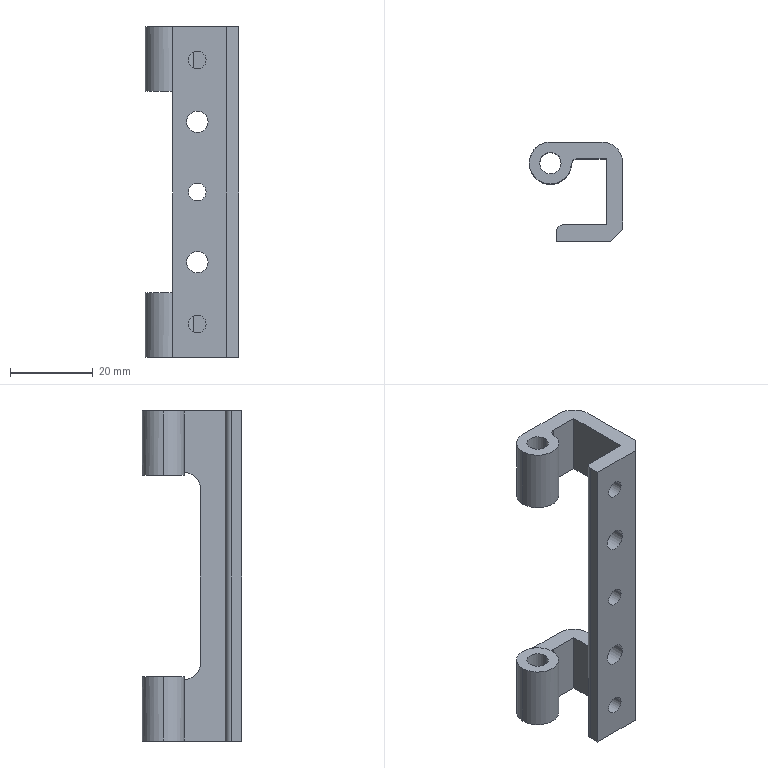Part | SolidWorks | features BaseBody 1 | 1 solid | 42 faces | box 22.6 x 24.1 x 80 mm | volume 10922 mm3 | cylinder 25 | plane 17 | commonest cylinder face diameters 5.2 x8 4.2 x6 10.2 x4 3 x3 8 x2 10 x2
STEP:
#1=CARTESIAN_POINT('',(8.6,0.,-17.));
#2=VERTEX_POINT('',#1);
#3=CARTESIAN_POINT('',(8.6,4.,-17.));
#4=VERTEX_POINT('',#3);
#5=CARTESIAN_POINT('',(8.6,-6.,-17.));
#6=DIRECTION('',(0.,1.,0.));
#7=VECTOR('',#6,1000.);
#8=LINE('',#5,#7);
#9=EDGE_CURVE('',#2,#4,#8,.T.);
#10=ORIENTED_EDGE('',*,*,#9,.F.);
#11=CARTESIAN_POINT('',(3.4,0.,-17.));
#12=VERTEX_POINT('',#11);
#13=CARTESIAN_POINT('',(6.,0.,-17.));
#14=DIRECTION('',(0.,1.,0.));
#15=DIRECTION('',(0.,0.,1.));
#16=AXIS2_PLACEMENT_3D('',#13,#14,#15);
#17=CIRCLE('',#16,2.6);
#18=EDGE_CURVE('',#12,#2,#17,.T.);
#19=ORIENTED_EDGE('',*,*,#18,.F.);
#20=CARTESIAN_POINT('',(3.4,4.,-17.));
#21=VERTEX_POINT('',#20);
#22=CARTESIAN_POINT('',(3.4,-6.,-17.));
#23=DIRECTION('',(0.,1.,0.));
#24=VECTOR('',#23,1000.);
#25=LINE('',#22,#24);
#26=EDGE_CURVE('',#12,#21,#25,.T.);
#27=ORIENTED_EDGE('',*,*,#26,.T.);
#28=CARTESIAN_POINT('',(6.,4.,-17.));
#29=DIRECTION('',(0.,1.,0.));
#30=DIRECTION('',(-1.,0.,0.));
#31=AXIS2_PLACEMENT_3D('',#28,#29,#30);
#32=CIRCLE('',#31,2.6);
#33=EDGE_CURVE('',#21,#4,#32,.T.);
#34=ORIENTED_EDGE('',*,*,#33,.T.);
#35=EDGE_LOOP('',(#10,#19,#27,#34));
#36=FACE_OUTER_BOUND('',#35,.T.);
#37=CARTESIAN_POINT('',(6.,-6.,-17.));
#38=DIRECTION('',(0.,1.,0.));
#39=DIRECTION('',(-1.,0.,0.));
#40=AXIS2_PLACEMENT_3D('',#37,#38,#39);
#41=CYLINDRICAL_SURFACE('',#40,2.6);
#42=ADVANCED_FACE('',(#36),#41,.F.);
#43=CARTESIAN_POINT('',(8.6,0.,17.));
#44=VERTEX_POINT('',#43);
#45=CARTESIAN_POINT('',(8.6,4.,17.));
#46=VERTEX_POINT('',#45);
#47=CARTESIAN_POINT('',(8.6,-6.,17.));
#48=DIRECTION('',(0.,1.,0.));
#49=VECTOR('',#48,1000.);
#50=LINE('',#47,#49);
#51=EDGE_CURVE('',#44,#46,#50,.T.);
#52=ORIENTED_EDGE('',*,*,#51,.F.);
#53=CARTESIAN_POINT('',(3.4,0.,17.));
#54=VERTEX_POINT('',#53);
#55=CARTESIAN_POINT('',(6.,0.,17.));
#56=DIRECTION('',(0.,1.,0.));
#57=DIRECTION('',(0.,0.,1.));
#58=AXIS2_PLACEMENT_3D('',#55,#56,#57);
#59=CIRCLE('',#58,2.6);
#60=EDGE_CURVE('',#54,#44,#59,.T.);
#61=ORIENTED_EDGE('',*,*,#60,.F.);
#62=CARTESIAN_POINT('',(3.4,4.,17.));
#63=VERTEX_POINT('',#62);
#64=CARTESIAN_POINT('',(3.4,-6.,17.));
#65=DIRECTION('',(0.,1.,0.));
#66=VECTOR('',#65,1000.);
#67=LINE('',#64,#66);
#68=EDGE_CURVE('',#54,#63,#67,.T.);
#69=ORIENTED_EDGE('',*,*,#68,.T.);
#70=CARTESIAN_POINT('',(6.,4.,17.));
#71=DIRECTION('',(0.,1.,0.));
#72=DIRECTION('',(-1.,0.,0.));
#73=AXIS2_PLACEMENT_3D('',#70,#71,#72);
#74=CIRCLE('',#73,2.6);
#75=EDGE_CURVE('',#63,#46,#74,.T.);
#76=ORIENTED_EDGE('',*,*,#75,.T.);
#77=EDGE_LOOP('',(#52,#61,#69,#76));
#78=FACE_OUTER_BOUND('',#77,.T.);
#79=CARTESIAN_POINT('',(6.,-6.,17.));
#80=DIRECTION('',(0.,1.,0.));
#81=DIRECTION('',(-1.,0.,0.));
#82=AXIS2_PLACEMENT_3D('',#79,#80,#81);
#83=CYLINDRICAL_SURFACE('',#82,2.6);
#84=ADVANCED_FACE('',(#78),#83,.F.);
#85=CARTESIAN_POINT('',(8.1,0.,-32.));
#86=VERTEX_POINT('',#85);
#87=CARTESIAN_POINT('',(8.1,4.,-32.));
#88=VERTEX_POINT('',#87);
#89=CARTESIAN_POINT('',(8.1,-6.,-32.));
#90=DIRECTION('',(0.,1.,0.));
#91=VECTOR('',#90,1000.);
#92=LINE('',#89,#91);
#93=EDGE_CURVE('',#86,#88,#92,.T.);
#94=ORIENTED_EDGE('',*,*,#93,.F.);
#95=CARTESIAN_POINT('',(3.9,0.,-32.));
#96=VERTEX_POINT('',#95);
#97=CARTESIAN_POINT('',(6.,0.,-32.));
#98=DIRECTION('',(0.,1.,0.));
#99=DIRECTION('',(0.,0.,1.));
#100=AXIS2_PLACEMENT_3D('',#97,#98,#99);
#101=CIRCLE('',#100,2.1);
#102=EDGE_CURVE('',#96,#86,#101,.T.);
#103=ORIENTED_EDGE('',*,*,#102,.F.);
#104=CARTESIAN_POINT('',(3.9,4.,-32.));
#105=VERTEX_POINT('',#104);
#106=CARTESIAN_POINT('',(3.9,-6.,-32.));
#107=DIRECTION('',(0.,1.,0.));
#108=VECTOR('',#107,1000.);
#109=LINE('',#106,#108);
#110=EDGE_CURVE('',#96,#105,#109,.T.);
#111=ORIENTED_EDGE('',*,*,#110,.T.);
#112=CARTESIAN_POINT('',(6.,4.,-32.));
#113=DIRECTION('',(0.,1.,0.));
#114=DIRECTION('',(-1.,0.,0.));
#115=AXIS2_PLACEMENT_3D('',#112,#113,#114);
#116=CIRCLE('',#115,2.1);
#117=EDGE_CURVE('',#105,#88,#116,.T.);
#118=ORIENTED_EDGE('',*,*,#117,.T.);
#119=EDGE_LOOP('',(#94,#103,#111,#118));
#120=FACE_OUTER_BOUND('',#119,.T.);
#121=CARTESIAN_POINT('',(6.,-6.,-32.));
#122=DIRECTION('',(0.,1.,0.));
#123=DIRECTION('',(-1.,0.,0.));
#124=AXIS2_PLACEMENT_3D('',#121,#122,#123);
#125=CYLINDRICAL_SURFACE('',#124,2.1);
#126=ADVANCED_FACE('',(#120),#125,.F.);
#127=CARTESIAN_POINT('',(8.1,0.,32.));
#128=VERTEX_POINT('',#127);
#129=CARTESIAN_POINT('',(8.1,4.,32.));
#130=VERTEX_POINT('',#129);
#131=CARTESIAN_POINT('',(8.1,-6.,32.));
#132=DIRECTION('',(0.,1.,0.));
#133=VECTOR('',#132,1000.);
#134=LINE('',#131,#133);
#135=EDGE_CURVE('',#128,#130,#134,.T.);
#136=ORIENTED_EDGE('',*,*,#135,.F.);
#137=CARTESIAN_POINT('',(3.9,0.,32.));
#138=VERTEX_POINT('',#137);
#139=CARTESIAN_POINT('',(6.,0.,32.));
#140=DIRECTION('',(0.,1.,0.));
#141=DIRECTION('',(0.,0.,1.));
#142=AXIS2_PLACEMENT_3D('',#139,#140,#141);
#143=CIRCLE('',#142,2.1);
#144=EDGE_CURVE('',#138,#128,#143,.T.);
#145=ORIENTED_EDGE('',*,*,#144,.F.);
#146=CARTESIAN_POINT('',(3.9,4.,32.));
#147=VERTEX_POINT('',#146);
#148=CARTESIAN_POINT('',(3.9,-6.,32.));
#149=DIRECTION('',(0.,1.,0.));
#150=VECTOR('',#149,1000.);
#151=LINE('',#148,#150);
#152=EDGE_CURVE('',#138,#147,#151,.T.);
#153=ORIENTED_EDGE('',*,*,#152,.T.);
#154=CARTESIAN_POINT('',(6.,4.,32.));
#155=DIRECTION('',(0.,1.,0.));
#156=DIRECTION('',(-1.,0.,0.));
#157=AXIS2_PLACEMENT_3D('',#154,#155,#156);
#158=CIRCLE('',#157,2.1);
#159=EDGE_CURVE('',#147,#130,#158,.T.);
#160=ORIENTED_EDGE('',*,*,#159,.T.);
#161=EDGE_LOOP('',(#136,#145,#153,#160));
#162=FACE_OUTER_BOUND('',#161,.T.);
#163=CARTESIAN_POINT('',(6.,-6.,32.));
#164=DIRECTION('',(0.,1.,0.));
#165=DIRECTION('',(-1.,0.,0.));
#166=AXIS2_PLACEMENT_3D('',#163,#164,#165);
#167=CYLINDRICAL_SURFACE('',#166,2.1);
#168=ADVANCED_FACE('',(#162),#167,.F.);
#169=CARTESIAN_POINT('',(8.1,0.,0.));
#170=VERTEX_POINT('',#169);
#171=CARTESIAN_POINT('',(8.1,4.,0.));
#172=VERTEX_POINT('',#171);
#173=CARTESIAN_POINT('',(8.1,-6.,0.));
#174=DIRECTION('',(0.,1.,0.));
#175=VECTOR('',#174,1000.);
#176=LINE('',#173,#175);
#177=EDGE_CURVE('',#170,#172,#176,.T.);
#178=ORIENTED_EDGE('',*,*,#177,.F.);
#179=CARTESIAN_POINT('',(3.9,0.,0.));
#180=VERTEX_POINT('',#179);
#181=CARTESIAN_POINT('',(6.,0.,0.));
#182=DIRECTION('',(0.,1.,0.));
#183=DIRECTION('',(0.,0.,1.));
#184=AXIS2_PLACEMENT_3D('',#181,#182,#183);
#185=CIRCLE('',#184,2.1);
#186=EDGE_CURVE('',#180,#170,#185,.T.);
#187=ORIENTED_EDGE('',*,*,#186,.F.);
#188=CARTESIAN_POINT('',(3.9,4.,0.));
#189=VERTEX_POINT('',#188);
#190=CARTESIAN_POINT('',(3.9,-6.,0.));
#191=DIRECTION('',(0.,1.,0.));
#192=VECTOR('',#191,1000.);
#193=LINE('',#190,#192);
#194=EDGE_CURVE('',#180,#189,#193,.T.);
#195=ORIENTED_EDGE('',*,*,#194,.T.);
#196=CARTESIAN_POINT('',(6.,4.,0.));
#197=DIRECTION('',(0.,1.,0.));
#198=DIRECTION('',(-1.,0.,0.));
#199=AXIS2_PLACEMENT_3D('',#196,#197,#198);
#200=CIRCLE('',#199,2.1);
#201=EDGE_CURVE('',#189,#172,#200,.T.);
#202=ORIENTED_EDGE('',*,*,#201,.T.);
#203=EDGE_LOOP('',(#178,#187,#195,#202));
#204=FACE_OUTER_BOUND('',#203,.T.);
#205=CARTESIAN_POINT('',(6.,-6.,0.));
#206=DIRECTION('',(0.,1.,0.));
#207=DIRECTION('',(-1.,0.,0.));
#208=AXIS2_PLACEMENT_3D('',#205,#206,#207);
#209=CYLINDRICAL_SURFACE('',#208,2.1);
#210=ADVANCED_FACE('',(#204),#209,.F.);
#211=CARTESIAN_POINT('',(13.,0.,40.));
#212=VERTEX_POINT('',#211);
#213=CARTESIAN_POINT('',(16.,3.,40.));
#214=VERTEX_POINT('',#213);
#215=CARTESIAN_POINT('',(15.25,2.25,40.));
#216=DIRECTION('',(0.7071,0.7071,0.));
#217=VECTOR('',#216,1000.);
#218=LINE('',#215,#217);
#219=EDGE_CURVE('',#212,#214,#218,.T.);
#220=ORIENTED_EDGE('',*,*,#219,.F.);
#221=CARTESIAN_POINT('',(13.,0.,-40.));
#222=VERTEX_POINT('',#221);
#223=CARTESIAN_POINT('',(13.,0.,40.));
#224=DIRECTION('',(0.,0.,1.));
#225=VECTOR('',#224,1000.);
#226=LINE('',#223,#225);
#227=EDGE_CURVE('',#222,#212,#226,.T.);
#228=ORIENTED_EDGE('',*,*,#227,.F.);
#229=CARTESIAN_POINT('',(16.,3.,-40.));
#230=VERTEX_POINT('',#229);
#231=CARTESIAN_POINT('',(16.,3.,-40.));
#232=DIRECTION('',(-0.7071,-0.7071,0.));
#233=VECTOR('',#232,1000.);
#234=LINE('',#231,#233);
#235=EDGE_CURVE('',#230,#222,#234,.T.);
#236=ORIENTED_EDGE('',*,*,#235,.F.);
#237=CARTESIAN_POINT('',(16.,3.,40.));
#238=DIRECTION('',(0.,0.,-1.));
#239=VECTOR('',#238,1000.);
#240=LINE('',#237,#239);
#241=EDGE_CURVE('',#214,#230,#240,.T.);
#242=ORIENTED_EDGE('',*,*,#241,.F.);
#243=EDGE_LOOP('',(#220,#228,#236,#242));
#244=FACE_OUTER_BOUND('',#243,.T.);
#245=CARTESIAN_POINT('',(16.,3.,40.));
#246=DIRECTION('',(-0.7071,0.7071,0.));
#247=DIRECTION('',(0.,0.,1.));
#248=AXIS2_PLACEMENT_3D('',#245,#246,#247);
#249=PLANE('',#248);
#250=ADVANCED_FACE('',(#244),#249,.F.);
#251=CARTESIAN_POINT('',(16.,14.,-25.1));
#252=VERTEX_POINT('',#251);
#253=CARTESIAN_POINT('',(16.,10.,-21.1));
#254=VERTEX_POINT('',#253);
#255=CARTESIAN_POINT('',(16.,14.,-21.1));
#256=DIRECTION('',(-1.,0.,0.));
#257=DIRECTION('',(0.,0.,1.));
#258=AXIS2_PLACEMENT_3D('',#255,#256,#257);
#259=CIRCLE('',#258,4.);
#260=EDGE_CURVE('',#252,#254,#259,.T.);
#261=ORIENTED_EDGE('',*,*,#260,.F.);
#262=CARTESIAN_POINT('',(12.,14.,-25.1));
#263=VERTEX_POINT('',#262);
#264=CARTESIAN_POINT('',(16.,14.,-25.1));
#265=DIRECTION('',(1.,0.,0.));
#266=VECTOR('',#265,1000.);
#267=LINE('',#264,#266);
#268=EDGE_CURVE('',#263,#252,#267,.T.);
#269=ORIENTED_EDGE('',*,*,#268,.F.);
#270=CARTESIAN_POINT('',(12.,10.,-21.1));
#271=VERTEX_POINT('',#270);
#272=CARTESIAN_POINT('',(12.,14.,-21.1));
#273=DIRECTION('',(1.,0.,0.));
#274=DIRECTION('',(0.,1.,0.));
#275=AXIS2_PLACEMENT_3D('',#272,#273,#274);
#276=CIRCLE('',#275,4.);
#277=EDGE_CURVE('',#271,#263,#276,.T.);
#278=ORIENTED_EDGE('',*,*,#277,.F.);
#279=CARTESIAN_POINT('',(0.,10.,-21.1));
#280=DIRECTION('',(-1.,0.,0.));
#281=VECTOR('',#280,1000.);
#282=LINE('',#279,#281);
#283=EDGE_CURVE('',#254,#271,#282,.T.);
#284=ORIENTED_EDGE('',*,*,#283,.F.);
#285=EDGE_LOOP('',(#261,#269,#278,#284));
#286=FACE_OUTER_BOUND('',#285,.T.);
#287=CARTESIAN_POINT('',(0.,14.,-21.1));
#288=DIRECTION('',(-1.,0.,0.));
#289=DIRECTION('',(0.,0.,1.));
#290=AXIS2_PLACEMENT_3D('',#287,#288,#289);
#291=CYLINDRICAL_SURFACE('',#290,4.);
#292=ADVANCED_FACE('',(#286),#291,.F.);
#293=CARTESIAN_POINT('',(12.,14.,25.1));
#294=VERTEX_POINT('',#293);
#295=CARTESIAN_POINT('',(12.,10.,21.1));
#296=VERTEX_POINT('',#295);
#297=CARTESIAN_POINT('',(12.,14.,21.1));
#298=DIRECTION('',(1.,0.,0.));
#299=DIRECTION('',(0.,1.,0.));
#300=AXIS2_PLACEMENT_3D('',#297,#298,#299);
#301=CIRCLE('',#300,4.);
#302=EDGE_CURVE('',#294,#296,#301,.T.);
#303=ORIENTED_EDGE('',*,*,#302,.F.);
#304=CARTESIAN_POINT('',(16.,14.,25.1));
#305=VERTEX_POINT('',#304);
#306=CARTESIAN_POINT('',(16.,14.,25.1));
#307=DIRECTION('',(-1.,0.,0.));
#308=VECTOR('',#307,1000.);
#309=LINE('',#306,#308);
#310=EDGE_CURVE('',#305,#294,#309,.T.);
#311=ORIENTED_EDGE('',*,*,#310,.F.);
#312=CARTESIAN_POINT('',(16.,10.,21.1));
#313=VERTEX_POINT('',#312);
#314=CARTESIAN_POINT('',(16.,14.,21.1));
#315=DIRECTION('',(-1.,0.,0.));
#316=DIRECTION('',(0.,0.,1.));
#317=AXIS2_PLACEMENT_3D('',#314,#315,#316);
#318=CIRCLE('',#317,4.);
#319=EDGE_CURVE('',#313,#305,#318,.T.);
#320=ORIENTED_EDGE('',*,*,#319,.F.);
#321=CARTESIAN_POINT('',(0.,10.,21.1));
#322=DIRECTION('',(1.,0.,0.));
#323=VECTOR('',#322,1000.);
#324=LINE('',#321,#323);
#325=EDGE_CURVE('',#296,#313,#324,.T.);
#326=ORIENTED_EDGE('',*,*,#325,.F.);
#327=EDGE_LOOP('',(#303,#311,#320,#326));
#328=FACE_OUTER_BOUND('',#327,.T.);
#329=CARTESIAN_POINT('',(0.,14.,21.1));
#330=DIRECTION('',(1.,0.,0.));
#331=DIRECTION('',(0.,0.,-1.));
#332=AXIS2_PLACEMENT_3D('',#329,#330,#331);
#333=CYLINDRICAL_SURFACE('',#332,4.);
#334=ADVANCED_FACE('',(#328),#333,.F.);
#335=CARTESIAN_POINT('',(-4.1,19.,-24.4));
#336=VERTEX_POINT('',#335);
#337=CARTESIAN_POINT('',(1.1,19.,-24.4));
#338=VERTEX_POINT('',#337);
#339=CARTESIAN_POINT('',(-1.5,19.,-24.4));
#340=DIRECTION('',(0.,0.,-1.));
#341=DIRECTION('',(-1.,0.,0.));
#342=AXIS2_PLACEMENT_3D('',#339,#340,#341);
#343=CIRCLE('',#342,2.6);
#344=EDGE_CURVE('',#336,#338,#343,.T.);
#345=ORIENTED_EDGE('',*,*,#344,.T.);
#346=CARTESIAN_POINT('',(-1.5,19.,-24.4));
#347=DIRECTION('',(0.,0.,-1.));
#348=DIRECTION('',(-1.,0.,0.));
#349=AXIS2_PLACEMENT_3D('',#346,#347,#348);
#350=CIRCLE('',#349,2.6);
#351=EDGE_CURVE('',#338,#336,#350,.T.);
#352=ORIENTED_EDGE('',*,*,#351,.T.);
#353=EDGE_LOOP('',(#345,#352));
#354=FACE_BOUND('',#353,.T.);
#355=CARTESIAN_POINT('',(-6.6,19.,-24.4));
#356=VERTEX_POINT('',#355);
#357=CARTESIAN_POINT('',(3.6,19.,-24.4));
#358=VERTEX_POINT('',#357);
#359=CARTESIAN_POINT('',(-1.5,19.,-24.4));
#360=DIRECTION('',(0.,0.,-1.));
#361=DIRECTION('',(-1.,0.,0.));
#362=AXIS2_PLACEMENT_3D('',#359,#360,#361);
#363=CIRCLE('',#362,5.1);
#364=EDGE_CURVE('',#356,#358,#363,.T.);
#365=ORIENTED_EDGE('',*,*,#364,.F.);
#366=CARTESIAN_POINT('',(-1.5,19.,-24.4));
#367=DIRECTION('',(0.,0.,-1.));
#368=DIRECTION('',(-1.,0.,0.));
#369=AXIS2_PLACEMENT_3D('',#366,#367,#368);
#370=CIRCLE('',#369,5.1);
#371=EDGE_CURVE('',#358,#356,#370,.T.);
#372=ORIENTED_EDGE('',*,*,#371,.F.);
#373=EDGE_LOOP('',(#365,#372));
#374=FACE_OUTER_BOUND('',#373,.T.);
#375=CARTESIAN_POINT('',(-1.5,19.,-24.4));
#376=DIRECTION('',(0.,0.,1.));
#377=DIRECTION('',(1.,0.,0.));
#378=AXIS2_PLACEMENT_3D('',#375,#376,#377);
#379=PLANE('',#378);
#380=ADVANCED_FACE('',(#354,#374),#379,.T.);
#381=CARTESIAN_POINT('',(-4.1,19.,24.4));
#382=VERTEX_POINT('',#381);
#383=CARTESIAN_POINT('',(1.1,19.,24.4));
#384=VERTEX_POINT('',#383);
#385=CARTESIAN_POINT('',(-1.5,19.,24.4));
#386=DIRECTION('',(0.,0.,-1.));
#387=DIRECTION('',(-1.,0.,0.));
#388=AXIS2_PLACEMENT_3D('',#385,#386,#387);
#389=CIRCLE('',#388,2.6);
#390=EDGE_CURVE('',#382,#384,#389,.T.);
#391=ORIENTED_EDGE('',*,*,#390,.F.);
#392=CARTESIAN_POINT('',(-1.5,19.,24.4));
#393=DIRECTION('',(0.,0.,-1.));
#394=DIRECTION('',(-1.,0.,0.));
#395=AXIS2_PLACEMENT_3D('',#392,#393,#394);
#396=CIRCLE('',#395,2.6);
#397=EDGE_CURVE('',#384,#382,#396,.T.);
#398=ORIENTED_EDGE('',*,*,#397,.F.);
#399=EDGE_LOOP('',(#391,#398));
#400=FACE_BOUND('',#399,.T.);
#401=CARTESIAN_POINT('',(-6.6,19.,24.4));
#402=VERTEX_POINT('',#401);
#403=CARTESIAN_POINT('',(3.6,19.,24.4));
#404=VERTEX_POINT('',#403);
#405=CARTESIAN_POINT('',(-1.5,19.,24.4));
#406=DIRECTION('',(0.,0.,-1.));
#407=DIRECTION('',(-1.,0.,0.));
#408=AXIS2_PLACEMENT_3D('',#405,#406,#407);
#409=CIRCLE('',#408,5.1);
#410=EDGE_CURVE('',#402,#404,#409,.T.);
#411=ORIENTED_EDGE('',*,*,#410,.T.);
#412=CARTESIAN_POINT('',(-1.5,19.,24.4));
#413=DIRECTION('',(0.,0.,-1.));
#414=DIRECTION('',(-1.,0.,0.));
#415=AXIS2_PLACEMENT_3D('',#412,#413,#414);
#416=CIRCLE('',#415,5.1);
#417=EDGE_CURVE('',#404,#402,#416,.T.);
#418=ORIENTED_EDGE('',*,*,#417,.T.);
#419=EDGE_LOOP('',(#411,#418));
#420=FACE_OUTER_BOUND('',#419,.T.);
#421=CARTESIAN_POINT('',(-1.5,19.,24.4));
#422=DIRECTION('',(0.,0.,-1.));
#423=DIRECTION('',(-1.,0.,0.));
#424=AXIS2_PLACEMENT_3D('',#421,#422,#423);
#425=PLANE('',#424);
#426=ADVANCED_FACE('',(#400,#420),#425,.T.);
#427=CARTESIAN_POINT('',(12.,20.1,-25.1));
#428=VERTEX_POINT('',#427);
#429=CARTESIAN_POINT('',(12.,20.1,-25.1));
#430=DIRECTION('',(0.,1.,0.));
#431=VECTOR('',#430,1000.);
#432=LINE('',#429,#431);
#433=EDGE_CURVE('',#263,#428,#432,.T.);
#434=ORIENTED_EDGE('',*,*,#433,.F.);
#435=ORIENTED_EDGE('',*,*,#268,.T.);
#436=CARTESIAN_POINT('',(16.,19.1,-25.1));
#437=VERTEX_POINT('',#436);
#438=CARTESIAN_POINT('',(16.,10.,-25.1));
#439=DIRECTION('',(0.,1.,0.));
#440=VECTOR('',#439,1000.);
#441=LINE('',#438,#440);
#442=EDGE_CURVE('',#252,#437,#441,.T.);
#443=ORIENTED_EDGE('',*,*,#442,.T.);
#444=CARTESIAN_POINT('',(11.,24.1,-25.1));
#445=VERTEX_POINT('',#444);
#446=CARTESIAN_POINT('',(11.,19.1,-25.1));
#447=DIRECTION('',(0.,0.,1.));
#448=DIRECTION('',(-1.,0.,0.));
#449=AXIS2_PLACEMENT_3D('',#446,#447,#448);
#450=CIRCLE('',#449,5.);
#451=EDGE_CURVE('',#437,#445,#450,.T.);
#452=ORIENTED_EDGE('',*,*,#451,.T.);
#453=CARTESIAN_POINT('',(-1.5,24.1,-25.1));
#454=VERTEX_POINT('',#453);
#455=CARTESIAN_POINT('',(16.,24.1,-25.1));
#456=DIRECTION('',(-1.,0.,0.));
#457=VECTOR('',#456,1000.);
#458=LINE('',#455,#457);
#459=EDGE_CURVE('',#445,#454,#458,.T.);
#460=ORIENTED_EDGE('',*,*,#459,.T.);
#461=CARTESIAN_POINT('',(3.6,19.,-25.1));
#462=VERTEX_POINT('',#461);
#463=CARTESIAN_POINT('',(-1.5,19.,-25.1));
#464=DIRECTION('',(0.,0.,-1.));
#465=DIRECTION('',(-1.,0.,0.));
#466=AXIS2_PLACEMENT_3D('',#463,#464,#465);
#467=CIRCLE('',#466,5.1);
#468=EDGE_CURVE('',#454,#462,#467,.T.);
#469=ORIENTED_EDGE('',*,*,#468,.T.);
#470=CARTESIAN_POINT('',(3.591,18.691,-25.1));
#471=VERTEX_POINT('',#470);
#472=CARTESIAN_POINT('',(-1.5,19.,-25.1));
#473=DIRECTION('',(0.,0.,-1.));
#474=DIRECTION('',(-1.,0.,0.));
#475=AXIS2_PLACEMENT_3D('',#472,#473,#474);
#476=CIRCLE('',#475,5.1);
#477=EDGE_CURVE('',#462,#471,#476,.T.);
#478=ORIENTED_EDGE('',*,*,#477,.T.);
#479=CARTESIAN_POINT('',(5.088,20.1,-25.1));
#480=VERTEX_POINT('',#479);
#481=CARTESIAN_POINT('',(5.088,18.6,-25.1));
#482=DIRECTION('',(0.,0.,1.));
#483=DIRECTION('',(-1.,0.,0.));
#484=AXIS2_PLACEMENT_3D('',#481,#482,#483);
#485=CIRCLE('',#484,1.5);
#486=EDGE_CURVE('',#480,#471,#485,.T.);
#487=ORIENTED_EDGE('',*,*,#486,.F.);
#488=CARTESIAN_POINT('',(12.,20.1,-25.1));
#489=DIRECTION('',(-1.,0.,0.));
#490=VECTOR('',#489,1000.);
#491=LINE('',#488,#490);
#492=EDGE_CURVE('',#428,#480,#491,.T.);
#493=ORIENTED_EDGE('',*,*,#492,.F.);
#494=EDGE_LOOP('',(#434,#435,#443,#452,#460,#469,#478,#487,#493));
#495=FACE_OUTER_BOUND('',#494,.T.);
#496=CARTESIAN_POINT('',(16.,10.,-25.1));
#497=DIRECTION('',(0.,0.,-1.));
#498=DIRECTION('',(-1.,0.,0.));
#499=AXIS2_PLACEMENT_3D('',#496,#497,#498);
#500=PLANE('',#499);
#501=ADVANCED_FACE('',(#495),#500,.F.);
#502=CARTESIAN_POINT('',(12.,10.,40.));
#503=DIRECTION('',(0.,0.,1.));
#504=VECTOR('',#503,1000.);
#505=LINE('',#502,#504);
#506=EDGE_CURVE('',#271,#296,#505,.T.);
#507=ORIENTED_EDGE('',*,*,#506,.T.);
#508=ORIENTED_EDGE('',*,*,#325,.T.);
#509=CARTESIAN_POINT('',(16.,10.,25.1));
#510=DIRECTION('',(0.,0.,-1.));
#511=VECTOR('',#510,1000.);
#512=LINE('',#509,#511);
#513=EDGE_CURVE('',#313,#254,#512,.T.);
#514=ORIENTED_EDGE('',*,*,#513,.T.);
#515=ORIENTED_EDGE('',*,*,#283,.T.);
#516=EDGE_LOOP('',(#507,#508,#514,#515));
#517=FACE_OUTER_BOUND('',#516,.T.);
#518=CARTESIAN_POINT('',(0.,10.,0.));
#519=DIRECTION('',(0.,1.,0.));
#520=DIRECTION('',(1.,0.,0.));
#521=AXIS2_PLACEMENT_3D('',#518,#519,#520);
#522=PLANE('',#521);
#523=ADVANCED_FACE('',(#517),#522,.T.);
#524=CARTESIAN_POINT('',(11.,24.1,25.1));
#525=VERTEX_POINT('',#524);
#526=CARTESIAN_POINT('',(16.,19.1,25.1));
#527=VERTEX_POINT('',#526);
#528=CARTESIAN_POINT('',(11.,19.1,25.1));
#529=DIRECTION('',(0.,0.,-1.));
#530=DIRECTION('',(1.,0.,0.));
#531=AXIS2_PLACEMENT_3D('',#528,#529,#530);
#532=CIRCLE('',#531,5.);
#533=EDGE_CURVE('',#525,#527,#532,.T.);
#534=ORIENTED_EDGE('',*,*,#533,.F.);
#535=CARTESIAN_POINT('',(11.,24.1,40.));
#536=VERTEX_POINT('',#535);
#537=CARTESIAN_POINT('',(11.,24.1,40.));
#538=DIRECTION('',(0.,0.,-1.));
#539=VECTOR('',#538,1000.);
#540=LINE('',#537,#539);
#541=EDGE_CURVE('',#536,#525,#540,.T.);
#542=ORIENTED_EDGE('',*,*,#541,.F.);
#543=CARTESIAN_POINT('',(16.,19.1,40.));
#544=VERTEX_POINT('',#543);
#545=CARTESIAN_POINT('',(11.,19.1,40.));
#546=DIRECTION('',(0.,0.,1.));
#547=DIRECTION('',(1.,0.,0.));
#548=AXIS2_PLACEMENT_3D('',#545,#546,#547);
#549=CIRCLE('',#548,5.);
#550=EDGE_CURVE('',#544,#536,#549,.T.);
#551=ORIENTED_EDGE('',*,*,#550,.F.);
#552=CARTESIAN_POINT('',(16.,19.1,40.));
#553=DIRECTION('',(0.,0.,1.));
#554=VECTOR('',#553,1000.);
#555=LINE('',#552,#554);
#556=EDGE_CURVE('',#527,#544,#555,.T.);
#557=ORIENTED_EDGE('',*,*,#556,.F.);
#558=EDGE_LOOP('',(#534,#542,#551,#557));
#559=FACE_OUTER_BOUND('',#558,.T.);
#560=CARTESIAN_POINT('',(11.,19.1,40.));
#561=DIRECTION('',(0.,0.,-1.));
#562=DIRECTION('',(-1.,0.,0.));
#563=AXIS2_PLACEMENT_3D('',#560,#561,#562);
#564=CYLINDRICAL_SURFACE('',#563,5.);
#565=ADVANCED_FACE('',(#559),#564,.T.);
#566=CARTESIAN_POINT('',(3.591,18.691,25.1));
#567=VERTEX_POINT('',#566);
#568=CARTESIAN_POINT('',(3.591,18.691,40.));
#569=VERTEX_POINT('',#568);
#570=CARTESIAN_POINT('',(3.591,18.691,40.));
#571=DIRECTION('',(0.,0.,1.));
#572=VECTOR('',#571,1000.);
#573=LINE('',#570,#572);
#574=EDGE_CURVE('',#567,#569,#573,.T.);
#575=ORIENTED_EDGE('',*,*,#574,.F.);
#576=CARTESIAN_POINT('',(5.088,20.1,25.1));
#577=VERTEX_POINT('',#576);
#578=CARTESIAN_POINT('',(5.088,18.6,25.1));
#579=DIRECTION('',(0.,0.,-1.));
#580=DIRECTION('',(1.,0.,0.));
#581=AXIS2_PLACEMENT_3D('',#578,#579,#580);
#582=CIRCLE('',#581,1.5);
#583=EDGE_CURVE('',#567,#577,#582,.T.);
#584=ORIENTED_EDGE('',*,*,#583,.T.);
#585=CARTESIAN_POINT('',(5.088,20.1,40.));
#586=VERTEX_POINT('',#585);
#587=CARTESIAN_POINT('',(5.088,20.1,-40.));
#588=DIRECTION('',(0.,0.,-1.));
#589=VECTOR('',#588,1000.);
#590=LINE('',#587,#589);
#591=EDGE_CURVE('',#586,#577,#590,.T.);
#592=ORIENTED_EDGE('',*,*,#591,.F.);
#593=CARTESIAN_POINT('',(5.088,18.6,40.));
#594=DIRECTION('',(0.,0.,-1.));
#595=DIRECTION('',(1.,0.,0.));
#596=AXIS2_PLACEMENT_3D('',#593,#594,#595);
#597=CIRCLE('',#596,1.5);
#598=EDGE_CURVE('',#569,#586,#597,.T.);
#599=ORIENTED_EDGE('',*,*,#598,.F.);
#600=EDGE_LOOP('',(#575,#584,#592,#599));
#601=FACE_OUTER_BOUND('',#600,.T.);
#602=CARTESIAN_POINT('',(5.088,18.6,40.));
#603=DIRECTION('',(0.,0.,-1.));
#604=DIRECTION('',(-1.,0.,0.));
#605=AXIS2_PLACEMENT_3D('',#602,#603,#604);
#606=CYLINDRICAL_SURFACE('',#605,1.5);
#607=ADVANCED_FACE('',(#601),#606,.F.);
#608=CARTESIAN_POINT('',(1.5,4.,40.));
#609=VERTEX_POINT('',#608);
#610=CARTESIAN_POINT('',(0.,2.5,40.));
#611=VERTEX_POINT('',#610);
#612=CARTESIAN_POINT('',(1.5,2.5,40.));
#613=DIRECTION('',(0.,0.,1.));
#614=DIRECTION('',(1.,0.,0.));
#615=AXIS2_PLACEMENT_3D('',#612,#613,#614);
#616=CIRCLE('',#615,1.5);
#617=EDGE_CURVE('',#609,#611,#616,.T.);
#618=ORIENTED_EDGE('',*,*,#617,.F.);
#619=CARTESIAN_POINT('',(1.5,4.,-40.));
#620=VERTEX_POINT('',#619);
#621=CARTESIAN_POINT('',(1.5,4.,40.));
#622=DIRECTION('',(0.,0.,1.));
#623=VECTOR('',#622,1000.);
#624=LINE('',#621,#623);
#625=EDGE_CURVE('',#620,#609,#624,.T.);
#626=ORIENTED_EDGE('',*,*,#625,.F.);
#627=CARTESIAN_POINT('',(0.,2.5,-40.));
#628=VERTEX_POINT('',#627);
#629=CARTESIAN_POINT('',(1.5,2.5,-40.));
#630=DIRECTION('',(0.,0.,-1.));
#631=DIRECTION('',(1.,0.,0.));
#632=AXIS2_PLACEMENT_3D('',#629,#630,#631);
#633=CIRCLE('',#632,1.5);
#634=EDGE_CURVE('',#628,#620,#633,.T.);
#635=ORIENTED_EDGE('',*,*,#634,.F.);
#636=CARTESIAN_POINT('',(0.,2.5,40.));
#637=DIRECTION('',(0.,0.,-1.));
#638=VECTOR('',#637,1000.);
#639=LINE('',#636,#638);
#640=EDGE_CURVE('',#611,#628,#639,.T.);
#641=ORIENTED_EDGE('',*,*,#640,.F.);
#642=EDGE_LOOP('',(#618,#626,#635,#641));
#643=FACE_OUTER_BOUND('',#642,.T.);
#644=CARTESIAN_POINT('',(1.5,2.5,40.));
#645=DIRECTION('',(0.,0.,-1.));
#646=DIRECTION('',(-1.,0.,0.));
#647=AXIS2_PLACEMENT_3D('',#644,#645,#646);
#648=CYLINDRICAL_SURFACE('',#647,1.5);
#649=ADVANCED_FACE('',(#643),#648,.T.);
#650=CARTESIAN_POINT('',(1.1,19.,40.));
#651=VERTEX_POINT('',#650);
#652=CARTESIAN_POINT('',(1.1,19.,40.));
#653=DIRECTION('',(0.,0.,-1.));
#654=VECTOR('',#653,1000.);
#655=LINE('',#652,#654);
#656=EDGE_CURVE('',#651,#384,#655,.T.);
#657=ORIENTED_EDGE('',*,*,#656,.F.);
#658=CARTESIAN_POINT('',(-4.1,19.,40.));
#659=VERTEX_POINT('',#658);
#660=CARTESIAN_POINT('',(-1.5,19.,40.));
#661=DIRECTION('',(0.,0.,1.));
#662=DIRECTION('',(1.,0.,0.));
#663=AXIS2_PLACEMENT_3D('',#660,#661,#662);
#664=CIRCLE('',#663,2.6);
#665=EDGE_CURVE('',#651,#659,#664,.T.);
#666=ORIENTED_EDGE('',*,*,#665,.T.);
#667=CARTESIAN_POINT('',(-4.1,19.,40.));
#668=DIRECTION('',(0.,0.,-1.));
#669=VECTOR('',#668,1000.);
#670=LINE('',#667,#669);
#671=EDGE_CURVE('',#659,#382,#670,.T.);
#672=ORIENTED_EDGE('',*,*,#671,.T.);
#673=ORIENTED_EDGE('',*,*,#390,.T.);
#674=EDGE_LOOP('',(#657,#666,#672,#673));
#675=FACE_OUTER_BOUND('',#674,.T.);
#676=CARTESIAN_POINT('',(-1.5,19.,40.));
#677=DIRECTION('',(0.,0.,-1.));
#678=DIRECTION('',(-1.,0.,0.));
#679=AXIS2_PLACEMENT_3D('',#676,#677,#678);
#680=CYLINDRICAL_SURFACE('',#679,2.6);
#681=ADVANCED_FACE('',(#675),#680,.F.);
#682=ORIENTED_EDGE('',*,*,#201,.F.);
#683=CARTESIAN_POINT('',(6.,4.,0.));
#684=DIRECTION('',(0.,1.,0.));
#685=DIRECTION('',(-1.,0.,0.));
#686=AXIS2_PLACEMENT_3D('',#683,#684,#685);
#687=CIRCLE('',#686,2.1);
#688=EDGE_CURVE('',#172,#189,#687,.T.);
#689=ORIENTED_EDGE('',*,*,#688,.F.);
#690=EDGE_LOOP('',(#682,#689));
#691=FACE_BOUND('',#690,.T.);
#692=ORIENTED_EDGE('',*,*,#159,.F.);
#693=CARTESIAN_POINT('',(6.,4.,32.));
#694=DIRECTION('',(0.,1.,0.));
#695=DIRECTION('',(-1.,0.,0.));
#696=AXIS2_PLACEMENT_3D('',#693,#694,#695);
#697=CIRCLE('',#696,2.1);
#698=EDGE_CURVE('',#130,#147,#697,.T.);
#699=ORIENTED_EDGE('',*,*,#698,.F.);
#700=EDGE_LOOP('',(#692,#699));
#701=FACE_BOUND('',#700,.T.);
#702=ORIENTED_EDGE('',*,*,#117,.F.);
#703=CARTESIAN_POINT('',(6.,4.,-32.));
#704=DIRECTION('',(0.,1.,0.));
#705=DIRECTION('',(-1.,0.,0.));
#706=AXIS2_PLACEMENT_3D('',#703,#704,#705);
#707=CIRCLE('',#706,2.1);
#708=EDGE_CURVE('',#88,#105,#707,.T.);
#709=ORIENTED_EDGE('',*,*,#708,.F.);
#710=EDGE_LOOP('',(#702,#709));
#711=FACE_BOUND('',#710,.T.);
#712=ORIENTED_EDGE('',*,*,#75,.F.);
#713=CARTESIAN_POINT('',(6.,4.,17.));
#714=DIRECTION('',(0.,1.,0.));
#715=DIRECTION('',(-1.,0.,0.));
#716=AXIS2_PLACEMENT_3D('',#713,#714,#715);
#717=CIRCLE('',#716,2.6);
#718=EDGE_CURVE('',#46,#63,#717,.T.);
#719=ORIENTED_EDGE('',*,*,#718,.F.);
#720=EDGE_LOOP('',(#712,#719));
#721=FACE_BOUND('',#720,.T.);
#722=ORIENTED_EDGE('',*,*,#33,.F.);
#723=CARTESIAN_POINT('',(6.,4.,-17.));
#724=DIRECTION('',(0.,1.,0.));
#725=DIRECTION('',(-1.,0.,0.));
#726=AXIS2_PLACEMENT_3D('',#723,#724,#725);
#727=CIRCLE('',#726,2.6);
#728=EDGE_CURVE('',#4,#21,#727,.T.);
#729=ORIENTED_EDGE('',*,*,#728,.F.);
#730=EDGE_LOOP('',(#722,#729));
#731=FACE_BOUND('',#730,.T.);
#732=CARTESIAN_POINT('',(12.,4.,-40.));
#733=VERTEX_POINT('',#732);
#734=CARTESIAN_POINT('',(12.,4.,-40.));
#735=DIRECTION('',(-1.,0.,0.));
#736=VECTOR('',#735,1000.);
#737=LINE('',#734,#736);
#738=EDGE_CURVE('',#733,#620,#737,.T.);
#739=ORIENTED_EDGE('',*,*,#738,.T.);
#740=ORIENTED_EDGE('',*,*,#625,.T.);
#741=CARTESIAN_POINT('',(12.,4.,40.));
#742=VERTEX_POINT('',#741);
#743=CARTESIAN_POINT('',(12.,4.,40.));
#744=DIRECTION('',(-1.,0.,0.));
#745=VECTOR('',#744,1000.);
#746=LINE('',#743,#745);
#747=EDGE_CURVE('',#742,#609,#746,.T.);
#748=ORIENTED_EDGE('',*,*,#747,.F.);
#749=CARTESIAN_POINT('',(12.,4.,40.));
#750=DIRECTION('',(0.,0.,-1.));
#751=VECTOR('',#750,1000.);
#752=LINE('',#749,#751);
#753=EDGE_CURVE('',#742,#733,#752,.T.);
#754=ORIENTED_EDGE('',*,*,#753,.T.);
#755=EDGE_LOOP('',(#739,#740,#748,#754));
#756=FACE_OUTER_BOUND('',#755,.T.);
#757=CARTESIAN_POINT('',(12.,4.,40.));
#758=DIRECTION('',(0.,-1.,0.));
#759=DIRECTION('',(0.,0.,-1.));
#760=AXIS2_PLACEMENT_3D('',#757,#758,#759);
#761=PLANE('',#760);
#762=ADVANCED_FACE('',(#691,#701,#711,#721,#731,#756),#761,.F.);
#763=ORIENTED_EDGE('',*,*,#506,.F.);
#764=ORIENTED_EDGE('',*,*,#277,.T.);
#765=ORIENTED_EDGE('',*,*,#433,.T.);
#766=CARTESIAN_POINT('',(12.,20.1,-40.));
#767=VERTEX_POINT('',#766);
#768=CARTESIAN_POINT('',(12.,20.1,40.));
#769=DIRECTION('',(0.,0.,-1.));
#770=VECTOR('',#769,1000.);
#771=LINE('',#768,#770);
#772=EDGE_CURVE('',#428,#767,#771,.T.);
#773=ORIENTED_EDGE('',*,*,#772,.T.);
#774=CARTESIAN_POINT('',(12.,20.1,-40.));
#775=DIRECTION('',(0.,-1.,0.));
#776=VECTOR('',#775,1000.);
#777=LINE('',#774,#776);
#778=EDGE_CURVE('',#767,#733,#777,.T.);
#779=ORIENTED_EDGE('',*,*,#778,.T.);
#780=ORIENTED_EDGE('',*,*,#753,.F.);
#781=CARTESIAN_POINT('',(12.,20.1,40.));
#782=VERTEX_POINT('',#781);
#783=CARTESIAN_POINT('',(12.,20.1,40.));
#784=DIRECTION('',(0.,-1.,0.));
#785=VECTOR('',#784,1000.);
#786=LINE('',#783,#785);
#787=EDGE_CURVE('',#782,#742,#786,.T.);
#788=ORIENTED_EDGE('',*,*,#787,.F.);
#789=CARTESIAN_POINT('',(12.,20.1,25.1));
#790=VERTEX_POINT('',#789);
#791=CARTESIAN_POINT('',(12.,20.1,40.));
#792=DIRECTION('',(0.,0.,-1.));
#793=VECTOR('',#792,1000.);
#794=LINE('',#791,#793);
#795=EDGE_CURVE('',#782,#790,#794,.T.);
#796=ORIENTED_EDGE('',*,*,#795,.T.);
#797=CARTESIAN_POINT('',(12.,20.1,25.1));
#798=DIRECTION('',(0.,-1.,0.));
#799=VECTOR('',#798,1000.);
#800=LINE('',#797,#799);
#801=EDGE_CURVE('',#790,#294,#800,.T.);
#802=ORIENTED_EDGE('',*,*,#801,.T.);
#803=ORIENTED_EDGE('',*,*,#302,.T.);
#804=EDGE_LOOP('',(#763,#764,#765,#773,#779,#780,#788,#796,#802,#803));
#805=FACE_OUTER_BOUND('',#804,.T.);
#806=CARTESIAN_POINT('',(12.,20.1,40.));
#807=DIRECTION('',(1.,0.,0.));
#808=DIRECTION('',(0.,1.,0.));
#809=AXIS2_PLACEMENT_3D('',#806,#807,#808);
#810=PLANE('',#809);
#811=ADVANCED_FACE('',(#805),#810,.F.);
#812=ORIENTED_EDGE('',*,*,#591,.T.);
#813=CARTESIAN_POINT('',(12.,20.1,25.1));
#814=DIRECTION('',(1.,0.,0.));
#815=VECTOR('',#814,1000.);
#816=LINE('',#813,#815);
#817=EDGE_CURVE('',#577,#790,#816,.T.);
#818=ORIENTED_EDGE('',*,*,#817,.T.);
#819=ORIENTED_EDGE('',*,*,#795,.F.);
#820=CARTESIAN_POINT('',(12.,20.1,40.));
#821=DIRECTION('',(1.,0.,0.));
#822=VECTOR('',#821,1000.);
#823=LINE('',#820,#822);
#824=EDGE_CURVE('',#586,#782,#823,.T.);
#825=ORIENTED_EDGE('',*,*,#824,.F.);
#826=EDGE_LOOP('',(#812,#818,#819,#825));
#827=FACE_OUTER_BOUND('',#826,.T.);
#828=CARTESIAN_POINT('',(12.,20.1,40.));
#829=DIRECTION('',(0.,1.,0.));
#830=DIRECTION('',(1.,0.,0.));
#831=AXIS2_PLACEMENT_3D('',#828,#829,#830);
#832=PLANE('',#831);
#833=ADVANCED_FACE('',(#827),#832,.F.);
#834=CARTESIAN_POINT('',(3.6,19.,25.1));
#835=VERTEX_POINT('',#834);
#836=CARTESIAN_POINT('',(3.6,19.,40.));
#837=DIRECTION('',(0.,0.,-1.));
#838=VECTOR('',#837,1000.);
#839=LINE('',#836,#838);
#840=EDGE_CURVE('',#835,#404,#839,.T.);
#841=ORIENTED_EDGE('',*,*,#840,.F.);
#842=CARTESIAN_POINT('',(-1.5,19.,25.1));
#843=DIRECTION('',(0.,0.,-1.));
#844=DIRECTION('',(-1.,0.,0.));
#845=AXIS2_PLACEMENT_3D('',#842,#843,#844);
#846=CIRCLE('',#845,5.1);
#847=EDGE_CURVE('',#835,#567,#846,.T.);
#848=ORIENTED_EDGE('',*,*,#847,.T.);
#849=ORIENTED_EDGE('',*,*,#574,.T.);
#850=CARTESIAN_POINT('',(-6.6,19.,40.));
#851=VERTEX_POINT('',#850);
#852=CARTESIAN_POINT('',(-1.5,19.,40.));
#853=DIRECTION('',(0.,0.,1.));
#854=DIRECTION('',(1.,0.,0.));
#855=AXIS2_PLACEMENT_3D('',#852,#853,#854);
#856=CIRCLE('',#855,5.1);
#857=EDGE_CURVE('',#851,#569,#856,.T.);
#858=ORIENTED_EDGE('',*,*,#857,.F.);
#859=CARTESIAN_POINT('',(-6.6,19.,40.));
#860=DIRECTION('',(0.,0.,-1.));
#861=VECTOR('',#860,1000.);
#862=LINE('',#859,#861);
#863=EDGE_CURVE('',#851,#402,#862,.T.);
#864=ORIENTED_EDGE('',*,*,#863,.T.);
#865=ORIENTED_EDGE('',*,*,#417,.F.);
#866=EDGE_LOOP('',(#841,#848,#849,#858,#864,#865));
#867=FACE_OUTER_BOUND('',#866,.T.);
#868=CARTESIAN_POINT('',(-1.5,19.,40.));
#869=DIRECTION('',(0.,0.,-1.));
#870=DIRECTION('',(-1.,0.,0.));
#871=AXIS2_PLACEMENT_3D('',#868,#869,#870);
#872=CYLINDRICAL_SURFACE('',#871,5.1);
#873=ADVANCED_FACE('',(#867),#872,.T.);
#874=ORIENTED_EDGE('',*,*,#541,.T.);
#875=CARTESIAN_POINT('',(-1.5,24.1,25.1));
#876=VERTEX_POINT('',#875);
#877=CARTESIAN_POINT('',(16.,24.1,25.1));
#878=DIRECTION('',(1.,0.,0.));
#879=VECTOR('',#878,1000.);
#880=LINE('',#877,#879);
#881=EDGE_CURVE('',#876,#525,#880,.T.);
#882=ORIENTED_EDGE('',*,*,#881,.F.);
#883=CARTESIAN_POINT('',(-1.5,24.1,40.));
#884=VERTEX_POINT('',#883);
#885=CARTESIAN_POINT('',(-1.5,24.1,40.));
#886=DIRECTION('',(0.,0.,-1.));
#887=VECTOR('',#886,1000.);
#888=LINE('',#885,#887);
#889=EDGE_CURVE('',#884,#876,#888,.T.);
#890=ORIENTED_EDGE('',*,*,#889,.F.);
#891=CARTESIAN_POINT('',(-1.5,24.1,40.));
#892=DIRECTION('',(-1.,0.,0.));
#893=VECTOR('',#892,1000.);
#894=LINE('',#891,#893);
#895=EDGE_CURVE('',#536,#884,#894,.T.);
#896=ORIENTED_EDGE('',*,*,#895,.F.);
#897=EDGE_LOOP('',(#874,#882,#890,#896));
#898=FACE_OUTER_BOUND('',#897,.T.);
#899=CARTESIAN_POINT('',(-1.5,24.1,40.));
#900=DIRECTION('',(0.,-1.,0.));
#901=DIRECTION('',(-1.,0.,0.));
#902=AXIS2_PLACEMENT_3D('',#899,#900,#901);
#903=PLANE('',#902);
#904=ADVANCED_FACE('',(#898),#903,.F.);
#905=CARTESIAN_POINT('',(16.,0.,40.));
#906=DIRECTION('',(0.,1.,0.));
#907=VECTOR('',#906,1000.);
#908=LINE('',#905,#907);
#909=EDGE_CURVE('',#214,#544,#908,.T.);
#910=ORIENTED_EDGE('',*,*,#909,.F.);
#911=ORIENTED_EDGE('',*,*,#241,.T.);
#912=CARTESIAN_POINT('',(16.,19.1,-40.));
#913=VERTEX_POINT('',#912);
#914=CARTESIAN_POINT('',(16.,0.,-40.));
#915=DIRECTION('',(0.,1.,0.));
#916=VECTOR('',#915,1000.);
#917=LINE('',#914,#916);
#918=EDGE_CURVE('',#230,#913,#917,.T.);
#919=ORIENTED_EDGE('',*,*,#918,.T.);
#920=CARTESIAN_POINT('',(16.,19.1,40.));
#921=DIRECTION('',(0.,0.,1.));
#922=VECTOR('',#921,1000.);
#923=LINE('',#920,#922);
#924=EDGE_CURVE('',#913,#437,#923,.T.);
#925=ORIENTED_EDGE('',*,*,#924,.T.);
#926=ORIENTED_EDGE('',*,*,#442,.F.);
#927=ORIENTED_EDGE('',*,*,#260,.T.);
#928=ORIENTED_EDGE('',*,*,#513,.F.);
#929=ORIENTED_EDGE('',*,*,#319,.T.);
#930=CARTESIAN_POINT('',(16.,10.,25.1));
#931=DIRECTION('',(0.,1.,0.));
#932=VECTOR('',#931,1000.);
#933=LINE('',#930,#932);
#934=EDGE_CURVE('',#305,#527,#933,.T.);
#935=ORIENTED_EDGE('',*,*,#934,.T.);
#936=ORIENTED_EDGE('',*,*,#556,.T.);
#937=EDGE_LOOP('',(#910,#911,#919,#925,#926,#927,#928,#929,#935,#936));
#938=FACE_OUTER_BOUND('',#937,.T.);
#939=CARTESIAN_POINT('',(16.,0.,40.));
#940=DIRECTION('',(-1.,0.,0.));
#941=DIRECTION('',(0.,1.,0.));
#942=AXIS2_PLACEMENT_3D('',#939,#940,#941);
#943=PLANE('',#942);
#944=ADVANCED_FACE('',(#938),#943,.F.);
#945=ORIENTED_EDGE('',*,*,#186,.T.);
#946=CARTESIAN_POINT('',(6.,0.,0.));
#947=DIRECTION('',(0.,1.,0.));
#948=DIRECTION('',(0.,0.,1.));
#949=AXIS2_PLACEMENT_3D('',#946,#947,#948);
#950=CIRCLE('',#949,2.1);
#951=EDGE_CURVE('',#170,#180,#950,.T.);
#952=ORIENTED_EDGE('',*,*,#951,.T.);
#953=EDGE_LOOP('',(#945,#952));
#954=FACE_BOUND('',#953,.T.);
#955=ORIENTED_EDGE('',*,*,#144,.T.);
#956=CARTESIAN_POINT('',(6.,0.,32.));
#957=DIRECTION('',(0.,1.,0.));
#958=DIRECTION('',(0.,0.,1.));
#959=AXIS2_PLACEMENT_3D('',#956,#957,#958);
#960=CIRCLE('',#959,2.1);
#961=EDGE_CURVE('',#128,#138,#960,.T.);
#962=ORIENTED_EDGE('',*,*,#961,.T.);
#963=EDGE_LOOP('',(#955,#962));
#964=FACE_BOUND('',#963,.T.);
#965=ORIENTED_EDGE('',*,*,#102,.T.);
#966=CARTESIAN_POINT('',(6.,0.,-32.));
#967=DIRECTION('',(0.,1.,0.));
#968=DIRECTION('',(0.,0.,1.));
#969=AXIS2_PLACEMENT_3D('',#966,#967,#968);
#970=CIRCLE('',#969,2.1);
#971=EDGE_CURVE('',#86,#96,#970,.T.);
#972=ORIENTED_EDGE('',*,*,#971,.T.);
#973=EDGE_LOOP('',(#965,#972));
#974=FACE_BOUND('',#973,.T.);
#975=ORIENTED_EDGE('',*,*,#60,.T.);
#976=CARTESIAN_POINT('',(6.,0.,17.));
#977=DIRECTION('',(0.,1.,0.));
#978=DIRECTION('',(0.,0.,1.));
#979=AXIS2_PLACEMENT_3D('',#976,#977,#978);
#980=CIRCLE('',#979,2.6);
#981=EDGE_CURVE('',#44,#54,#980,.T.);
#982=ORIENTED_EDGE('',*,*,#981,.T.);
#983=EDGE_LOOP('',(#975,#982));
#984=FACE_BOUND('',#983,.T.);
#985=ORIENTED_EDGE('',*,*,#18,.T.);
#986=CARTESIAN_POINT('',(6.,0.,-17.));
#987=DIRECTION('',(0.,1.,0.));
#988=DIRECTION('',(0.,0.,1.));
#989=AXIS2_PLACEMENT_3D('',#986,#987,#988);
#990=CIRCLE('',#989,2.6);
#991=EDGE_CURVE('',#2,#12,#990,.T.);
#992=ORIENTED_EDGE('',*,*,#991,.T.);
#993=EDGE_LOOP('',(#985,#992));
#994=FACE_BOUND('',#993,.T.);
#995=CARTESIAN_POINT('',(0.,0.,-40.));
#996=VERTEX_POINT('',#995);
#997=CARTESIAN_POINT('',(0.,0.,-40.));
#998=DIRECTION('',(1.,0.,0.));
#999=VECTOR('',#998,1000.);
#1000=LINE('',#997,#999);
#1001=EDGE_CURVE('',#996,#222,#1000,.T.);
#1002=ORIENTED_EDGE('',*,*,#1001,.T.);
#1003=ORIENTED_EDGE('',*,*,#227,.T.);
#1004=CARTESIAN_POINT('',(0.,0.,40.));
#1005=VERTEX_POINT('',#1004);
#1006=CARTESIAN_POINT('',(0.,0.,40.));
#1007=DIRECTION('',(1.,0.,0.));
#1008=VECTOR('',#1007,1000.);
#1009=LINE('',#1006,#1008);
#1010=EDGE_CURVE('',#1005,#212,#1009,.T.);
#1011=ORIENTED_EDGE('',*,*,#1010,.F.);
#1012=CARTESIAN_POINT('',(0.,0.,40.));
#1013=DIRECTION('',(0.,0.,-1.));
#1014=VECTOR('',#1013,1000.);
#1015=LINE('',#1012,#1014);
#1016=EDGE_CURVE('',#1005,#996,#1015,.T.);
#1017=ORIENTED_EDGE('',*,*,#1016,.T.);
#1018=EDGE_LOOP('',(#1002,#1003,#1011,#1017));
#1019=FACE_OUTER_BOUND('',#1018,.T.);
#1020=CARTESIAN_POINT('',(0.,0.,40.));
#1021=DIRECTION('',(0.,1.,0.));
#1022=DIRECTION('',(1.,0.,0.));
#1023=AXIS2_PLACEMENT_3D('',#1020,#1021,#1022);
#1024=PLANE('',#1023);
#1025=ADVANCED_FACE('',(#954,#964,#974,#984,#994,#1019),#1024,.F.);
#1026=CARTESIAN_POINT('',(0.,4.,40.));
#1027=DIRECTION('',(0.,-1.,0.));
#1028=VECTOR('',#1027,1000.);
#1029=LINE('',#1026,#1028);
#1030=EDGE_CURVE('',#611,#1005,#1029,.T.);
#1031=ORIENTED_EDGE('',*,*,#1030,.F.);
#1032=ORIENTED_EDGE('',*,*,#640,.T.);
#1033=CARTESIAN_POINT('',(0.,4.,-40.));
#1034=DIRECTION('',(0.,-1.,0.));
#1035=VECTOR('',#1034,1000.);
#1036=LINE('',#1033,#1035);
#1037=EDGE_CURVE('',#628,#996,#1036,.T.);
#1038=ORIENTED_EDGE('',*,*,#1037,.T.);
#1039=ORIENTED_EDGE('',*,*,#1016,.F.);
#1040=EDGE_LOOP('',(#1031,#1032,#1038,#1039));
#1041=FACE_OUTER_BOUND('',#1040,.T.);
#1042=CARTESIAN_POINT('',(0.,4.,40.));
#1043=DIRECTION('',(1.,0.,0.));
#1044=DIRECTION('',(0.,1.,0.));
#1045=AXIS2_PLACEMENT_3D('',#1042,#1043,#1044);
#1046=PLANE('',#1045);
#1047=ADVANCED_FACE('',(#1041),#1046,.F.);
#1048=CARTESIAN_POINT('',(-4.1,19.,-40.));
#1049=VERTEX_POINT('',#1048);
#1050=CARTESIAN_POINT('',(1.1,19.,-40.));
#1051=VERTEX_POINT('',#1050);
#1052=CARTESIAN_POINT('',(-1.5,19.,-40.));
#1053=DIRECTION('',(0.,0.,1.));
#1054=DIRECTION('',(1.,0.,0.));
#1055=AXIS2_PLACEMENT_3D('',#1052,#1053,#1054);
#1056=CIRCLE('',#1055,2.6);
#1057=EDGE_CURVE('',#1049,#1051,#1056,.T.);
#1058=ORIENTED_EDGE('',*,*,#1057,.T.);
#1059=CARTESIAN_POINT('',(-1.5,19.,-40.));
#1060=DIRECTION('',(0.,0.,1.));
#1061=DIRECTION('',(1.,0.,0.));
#1062=AXIS2_PLACEMENT_3D('',#1059,#1060,#1061);
#1063=CIRCLE('',#1062,2.6);
#1064=EDGE_CURVE('',#1051,#1049,#1063,.T.);
#1065=ORIENTED_EDGE('',*,*,#1064,.T.);
#1066=EDGE_LOOP('',(#1058,#1065));
#1067=FACE_BOUND('',#1066,.T.);
#1068=ORIENTED_EDGE('',*,*,#918,.F.);
#1069=ORIENTED_EDGE('',*,*,#235,.T.);
#1070=ORIENTED_EDGE('',*,*,#1001,.F.);
#1071=ORIENTED_EDGE('',*,*,#1037,.F.);
#1072=ORIENTED_EDGE('',*,*,#634,.T.);
#1073=ORIENTED_EDGE('',*,*,#738,.F.);
#1074=ORIENTED_EDGE('',*,*,#778,.F.);
#1075=CARTESIAN_POINT('',(5.088,20.1,-40.));
#1076=VERTEX_POINT('',#1075);
#1077=CARTESIAN_POINT('',(12.,20.1,-40.));
#1078=DIRECTION('',(1.,0.,0.));
#1079=VECTOR('',#1078,1000.);
#1080=LINE('',#1077,#1079);
#1081=EDGE_CURVE('',#1076,#767,#1080,.T.);
#1082=ORIENTED_EDGE('',*,*,#1081,.F.);
#1083=CARTESIAN_POINT('',(3.591,18.691,-40.));
#1084=VERTEX_POINT('',#1083);
#1085=CARTESIAN_POINT('',(5.088,18.6,-40.));
#1086=DIRECTION('',(0.,0.,1.));
#1087=DIRECTION('',(1.,0.,0.));
#1088=AXIS2_PLACEMENT_3D('',#1085,#1086,#1087);
#1089=CIRCLE('',#1088,1.5);
#1090=EDGE_CURVE('',#1076,#1084,#1089,.T.);
#1091=ORIENTED_EDGE('',*,*,#1090,.T.);
#1092=CARTESIAN_POINT('',(-6.6,19.,-40.));
#1093=VERTEX_POINT('',#1092);
#1094=CARTESIAN_POINT('',(-1.5,19.,-40.));
#1095=DIRECTION('',(0.,0.,1.));
#1096=DIRECTION('',(1.,0.,0.));
#1097=AXIS2_PLACEMENT_3D('',#1094,#1095,#1096);
#1098=CIRCLE('',#1097,5.1);
#1099=EDGE_CURVE('',#1093,#1084,#1098,.T.);
#1100=ORIENTED_EDGE('',*,*,#1099,.F.);
#1101=CARTESIAN_POINT('',(-1.5,24.1,-40.));
#1102=VERTEX_POINT('',#1101);
#1103=CARTESIAN_POINT('',(-1.5,19.,-40.));
#1104=DIRECTION('',(0.,0.,1.));
#1105=DIRECTION('',(1.,0.,0.));
#1106=AXIS2_PLACEMENT_3D('',#1103,#1104,#1105);
#1107=CIRCLE('',#1106,5.1);
#1108=EDGE_CURVE('',#1102,#1093,#1107,.T.);
#1109=ORIENTED_EDGE('',*,*,#1108,.F.);
#1110=CARTESIAN_POINT('',(11.,24.1,-40.));
#1111=VERTEX_POINT('',#1110);
#1112=CARTESIAN_POINT('',(-1.5,24.1,-40.));
#1113=DIRECTION('',(-1.,0.,0.));
#1114=VECTOR('',#1113,1000.);
#1115=LINE('',#1112,#1114);
#1116=EDGE_CURVE('',#1111,#1102,#1115,.T.);
#1117=ORIENTED_EDGE('',*,*,#1116,.F.);
#1118=CARTESIAN_POINT('',(11.,19.1,-40.));
#1119=DIRECTION('',(0.,0.,-1.));
#1120=DIRECTION('',(1.,0.,0.));
#1121=AXIS2_PLACEMENT_3D('',#1118,#1119,#1120);
#1122=CIRCLE('',#1121,5.);
#1123=EDGE_CURVE('',#1111,#913,#1122,.T.);
#1124=ORIENTED_EDGE('',*,*,#1123,.T.);
#1125=EDGE_LOOP('',(#1068,#1069,#1070,#1071,#1072,#1073,#1074,#1082,#1091,#1100,#1109,#1117,#1124));
#1126=FACE_OUTER_BOUND('',#1125,.T.);
#1127=CARTESIAN_POINT('',(-1.5,19.,-40.));
#1128=DIRECTION('',(0.,0.,1.));
#1129=DIRECTION('',(0.,-1.,0.));
#1130=AXIS2_PLACEMENT_3D('',#1127,#1128,#1129);
#1131=PLANE('',#1130);
#1132=ADVANCED_FACE('',(#1067,#1126),#1131,.F.);
#1133=CARTESIAN_POINT('',(-1.5,19.,40.));
#1134=DIRECTION('',(0.,0.,1.));
#1135=DIRECTION('',(1.,0.,0.));
#1136=AXIS2_PLACEMENT_3D('',#1133,#1134,#1135);
#1137=CIRCLE('',#1136,2.6);
#1138=EDGE_CURVE('',#659,#651,#1137,.T.);
#1139=ORIENTED_EDGE('',*,*,#1138,.F.);
#1140=ORIENTED_EDGE('',*,*,#665,.F.);
#1141=EDGE_LOOP('',(#1139,#1140));
#1142=FACE_BOUND('',#1141,.T.);
#1143=ORIENTED_EDGE('',*,*,#1010,.T.);
#1144=ORIENTED_EDGE('',*,*,#219,.T.);
#1145=ORIENTED_EDGE('',*,*,#909,.T.);
#1146=ORIENTED_EDGE('',*,*,#550,.T.);
#1147=ORIENTED_EDGE('',*,*,#895,.T.);
#1148=CARTESIAN_POINT('',(-1.5,19.,40.));
#1149=DIRECTION('',(0.,0.,1.));
#1150=DIRECTION('',(1.,0.,0.));
#1151=AXIS2_PLACEMENT_3D('',#1148,#1149,#1150);
#1152=CIRCLE('',#1151,5.1);
#1153=EDGE_CURVE('',#884,#851,#1152,.T.);
#1154=ORIENTED_EDGE('',*,*,#1153,.T.);
#1155=ORIENTED_EDGE('',*,*,#857,.T.);
#1156=ORIENTED_EDGE('',*,*,#598,.T.);
#1157=ORIENTED_EDGE('',*,*,#824,.T.);
#1158=ORIENTED_EDGE('',*,*,#787,.T.);
#1159=ORIENTED_EDGE('',*,*,#747,.T.);
#1160=ORIENTED_EDGE('',*,*,#617,.T.);
#1161=ORIENTED_EDGE('',*,*,#1030,.T.);
#1162=EDGE_LOOP('',(#1143,#1144,#1145,#1146,#1147,#1154,#1155,#1156,#1157,#1158,#1159,#1160,#1161));
#1163=FACE_OUTER_BOUND('',#1162,.T.);
#1164=CARTESIAN_POINT('',(-1.5,19.,40.));
#1165=DIRECTION('',(0.,0.,1.));
#1166=DIRECTION('',(0.,-1.,0.));
#1167=AXIS2_PLACEMENT_3D('',#1164,#1165,#1166);
#1168=PLANE('',#1167);
#1169=ADVANCED_FACE('',(#1142,#1163),#1168,.T.);
#1170=ORIENTED_EDGE('',*,*,#451,.F.);
#1171=ORIENTED_EDGE('',*,*,#924,.F.);
#1172=ORIENTED_EDGE('',*,*,#1123,.F.);
#1173=CARTESIAN_POINT('',(11.,24.1,40.));
#1174=DIRECTION('',(0.,0.,-1.));
#1175=VECTOR('',#1174,1000.);
#1176=LINE('',#1173,#1175);
#1177=EDGE_CURVE('',#445,#1111,#1176,.T.);
#1178=ORIENTED_EDGE('',*,*,#1177,.F.);
#1179=EDGE_LOOP('',(#1170,#1171,#1172,#1178));
#1180=FACE_OUTER_BOUND('',#1179,.T.);
#1181=CARTESIAN_POINT('',(11.,19.1,40.));
#1182=DIRECTION('',(0.,0.,-1.));
#1183=DIRECTION('',(-1.,0.,0.));
#1184=AXIS2_PLACEMENT_3D('',#1181,#1182,#1183);
#1185=CYLINDRICAL_SURFACE('',#1184,5.);
#1186=ADVANCED_FACE('',(#1180),#1185,.T.);
#1187=CARTESIAN_POINT('',(5.088,20.1,-40.));
#1188=DIRECTION('',(0.,0.,-1.));
#1189=VECTOR('',#1188,1000.);
#1190=LINE('',#1187,#1189);
#1191=EDGE_CURVE('',#480,#1076,#1190,.T.);
#1192=ORIENTED_EDGE('',*,*,#1191,.F.);
#1193=ORIENTED_EDGE('',*,*,#486,.T.);
#1194=CARTESIAN_POINT('',(3.591,18.691,40.));
#1195=DIRECTION('',(0.,0.,1.));
#1196=VECTOR('',#1195,1000.);
#1197=LINE('',#1194,#1196);
#1198=EDGE_CURVE('',#1084,#471,#1197,.T.);
#1199=ORIENTED_EDGE('',*,*,#1198,.F.);
#1200=ORIENTED_EDGE('',*,*,#1090,.F.);
#1201=EDGE_LOOP('',(#1192,#1193,#1199,#1200));
#1202=FACE_OUTER_BOUND('',#1201,.T.);
#1203=CARTESIAN_POINT('',(5.088,18.6,40.));
#1204=DIRECTION('',(0.,0.,-1.));
#1205=DIRECTION('',(-1.,0.,0.));
#1206=AXIS2_PLACEMENT_3D('',#1203,#1204,#1205);
#1207=CYLINDRICAL_SURFACE('',#1206,1.5);
#1208=ADVANCED_FACE('',(#1202),#1207,.F.);
#1209=CARTESIAN_POINT('',(1.1,19.,40.));
#1210=DIRECTION('',(0.,0.,-1.));
#1211=VECTOR('',#1210,1000.);
#1212=LINE('',#1209,#1211);
#1213=EDGE_CURVE('',#338,#1051,#1212,.T.);
#1214=ORIENTED_EDGE('',*,*,#1213,.F.);
#1215=ORIENTED_EDGE('',*,*,#344,.F.);
#1216=CARTESIAN_POINT('',(-4.1,19.,40.));
#1217=DIRECTION('',(0.,0.,-1.));
#1218=VECTOR('',#1217,1000.);
#1219=LINE('',#1216,#1218);
#1220=EDGE_CURVE('',#336,#1049,#1219,.T.);
#1221=ORIENTED_EDGE('',*,*,#1220,.T.);
#1222=ORIENTED_EDGE('',*,*,#1064,.F.);
#1223=EDGE_LOOP('',(#1214,#1215,#1221,#1222));
#1224=FACE_OUTER_BOUND('',#1223,.T.);
#1225=CARTESIAN_POINT('',(-1.5,19.,40.));
#1226=DIRECTION('',(0.,0.,-1.));
#1227=DIRECTION('',(-1.,0.,0.));
#1228=AXIS2_PLACEMENT_3D('',#1225,#1226,#1227);
#1229=CYLINDRICAL_SURFACE('',#1228,2.6);
#1230=ADVANCED_FACE('',(#1224),#1229,.F.);
#1231=ORIENTED_EDGE('',*,*,#772,.F.);
#1232=ORIENTED_EDGE('',*,*,#492,.T.);
#1233=ORIENTED_EDGE('',*,*,#1191,.T.);
#1234=ORIENTED_EDGE('',*,*,#1081,.T.);
#1235=EDGE_LOOP('',(#1231,#1232,#1233,#1234));
#1236=FACE_OUTER_BOUND('',#1235,.T.);
#1237=CARTESIAN_POINT('',(12.,20.1,40.));
#1238=DIRECTION('',(0.,1.,0.));
#1239=DIRECTION('',(1.,0.,0.));
#1240=AXIS2_PLACEMENT_3D('',#1237,#1238,#1239);
#1241=PLANE('',#1240);
#1242=ADVANCED_FACE('',(#1236),#1241,.F.);
#1243=CARTESIAN_POINT('',(3.6,19.,40.));
#1244=DIRECTION('',(0.,0.,-1.));
#1245=VECTOR('',#1244,1000.);
#1246=LINE('',#1243,#1245);
#1247=EDGE_CURVE('',#358,#462,#1246,.T.);
#1248=ORIENTED_EDGE('',*,*,#1247,.F.);
#1249=ORIENTED_EDGE('',*,*,#371,.T.);
#1250=CARTESIAN_POINT('',(-6.6,19.,40.));
#1251=DIRECTION('',(0.,0.,-1.));
#1252=VECTOR('',#1251,1000.);
#1253=LINE('',#1250,#1252);
#1254=EDGE_CURVE('',#356,#1093,#1253,.T.);
#1255=ORIENTED_EDGE('',*,*,#1254,.T.);
#1256=ORIENTED_EDGE('',*,*,#1099,.T.);
#1257=ORIENTED_EDGE('',*,*,#1198,.T.);
#1258=ORIENTED_EDGE('',*,*,#477,.F.);
#1259=EDGE_LOOP('',(#1248,#1249,#1255,#1256,#1257,#1258));
#1260=FACE_OUTER_BOUND('',#1259,.T.);
#1261=CARTESIAN_POINT('',(-1.5,19.,40.));
#1262=DIRECTION('',(0.,0.,-1.));
#1263=DIRECTION('',(-1.,0.,0.));
#1264=AXIS2_PLACEMENT_3D('',#1261,#1262,#1263);
#1265=CYLINDRICAL_SURFACE('',#1264,5.1);
#1266=ADVANCED_FACE('',(#1260),#1265,.T.);
#1267=CARTESIAN_POINT('',(-1.5,24.1,40.));
#1268=DIRECTION('',(0.,0.,-1.));
#1269=VECTOR('',#1268,1000.);
#1270=LINE('',#1267,#1269);
#1271=EDGE_CURVE('',#454,#1102,#1270,.T.);
#1272=ORIENTED_EDGE('',*,*,#1271,.F.);
#1273=ORIENTED_EDGE('',*,*,#459,.F.);
#1274=ORIENTED_EDGE('',*,*,#1177,.T.);
#1275=ORIENTED_EDGE('',*,*,#1116,.T.);
#1276=EDGE_LOOP('',(#1272,#1273,#1274,#1275));
#1277=FACE_OUTER_BOUND('',#1276,.T.);
#1278=CARTESIAN_POINT('',(-1.5,24.1,40.));
#1279=DIRECTION('',(0.,-1.,0.));
#1280=DIRECTION('',(-1.,0.,0.));
#1281=AXIS2_PLACEMENT_3D('',#1278,#1279,#1280);
#1282=PLANE('',#1281);
#1283=ADVANCED_FACE('',(#1277),#1282,.F.);
#1284=ORIENTED_EDGE('',*,*,#934,.F.);
#1285=ORIENTED_EDGE('',*,*,#310,.T.);
#1286=ORIENTED_EDGE('',*,*,#801,.F.);
#1287=ORIENTED_EDGE('',*,*,#817,.F.);
#1288=ORIENTED_EDGE('',*,*,#583,.F.);
#1289=ORIENTED_EDGE('',*,*,#847,.F.);
#1290=CARTESIAN_POINT('',(-1.5,19.,25.1));
#1291=DIRECTION('',(0.,0.,-1.));
#1292=DIRECTION('',(-1.,0.,0.));
#1293=AXIS2_PLACEMENT_3D('',#1290,#1291,#1292);
#1294=CIRCLE('',#1293,5.1);
#1295=EDGE_CURVE('',#876,#835,#1294,.T.);
#1296=ORIENTED_EDGE('',*,*,#1295,.F.);
#1297=ORIENTED_EDGE('',*,*,#881,.T.);
#1298=ORIENTED_EDGE('',*,*,#533,.T.);
#1299=EDGE_LOOP('',(#1284,#1285,#1286,#1287,#1288,#1289,#1296,#1297,#1298));
#1300=FACE_OUTER_BOUND('',#1299,.T.);
#1301=CARTESIAN_POINT('',(16.,10.,25.1));
#1302=DIRECTION('',(0.,0.,1.));
#1303=DIRECTION('',(1.,0.,0.));
#1304=AXIS2_PLACEMENT_3D('',#1301,#1302,#1303);
#1305=PLANE('',#1304);
#1306=ADVANCED_FACE('',(#1300),#1305,.F.);
#1307=ORIENTED_EDGE('',*,*,#364,.T.);
#1308=ORIENTED_EDGE('',*,*,#1247,.T.);
#1309=ORIENTED_EDGE('',*,*,#468,.F.);
#1310=ORIENTED_EDGE('',*,*,#1271,.T.);
#1311=ORIENTED_EDGE('',*,*,#1108,.T.);
#1312=ORIENTED_EDGE('',*,*,#1254,.F.);
#1313=EDGE_LOOP('',(#1307,#1308,#1309,#1310,#1311,#1312));
#1314=FACE_OUTER_BOUND('',#1313,.T.);
#1315=CARTESIAN_POINT('',(-1.5,19.,40.));
#1316=DIRECTION('',(0.,0.,-1.));
#1317=DIRECTION('',(-1.,0.,0.));
#1318=AXIS2_PLACEMENT_3D('',#1315,#1316,#1317);
#1319=CYLINDRICAL_SURFACE('',#1318,5.1);
#1320=ADVANCED_FACE('',(#1314),#1319,.T.);
#1321=ORIENTED_EDGE('',*,*,#351,.F.);
#1322=ORIENTED_EDGE('',*,*,#1213,.T.);
#1323=ORIENTED_EDGE('',*,*,#1057,.F.);
#1324=ORIENTED_EDGE('',*,*,#1220,.F.);
#1325=EDGE_LOOP('',(#1321,#1322,#1323,#1324));
#1326=FACE_OUTER_BOUND('',#1325,.T.);
#1327=CARTESIAN_POINT('',(-1.5,19.,40.));
#1328=DIRECTION('',(0.,0.,-1.));
#1329=DIRECTION('',(-1.,0.,0.));
#1330=AXIS2_PLACEMENT_3D('',#1327,#1328,#1329);
#1331=CYLINDRICAL_SURFACE('',#1330,2.6);
#1332=ADVANCED_FACE('',(#1326),#1331,.F.);
#1333=ORIENTED_EDGE('',*,*,#1295,.T.);
#1334=ORIENTED_EDGE('',*,*,#840,.T.);
#1335=ORIENTED_EDGE('',*,*,#410,.F.);
#1336=ORIENTED_EDGE('',*,*,#863,.F.);
#1337=ORIENTED_EDGE('',*,*,#1153,.F.);
#1338=ORIENTED_EDGE('',*,*,#889,.T.);
#1339=EDGE_LOOP('',(#1333,#1334,#1335,#1336,#1337,#1338));
#1340=FACE_OUTER_BOUND('',#1339,.T.);
#1341=CARTESIAN_POINT('',(-1.5,19.,40.));
#1342=DIRECTION('',(0.,0.,-1.));
#1343=DIRECTION('',(-1.,0.,0.));
#1344=AXIS2_PLACEMENT_3D('',#1341,#1342,#1343);
#1345=CYLINDRICAL_SURFACE('',#1344,5.1);
#1346=ADVANCED_FACE('',(#1340),#1345,.T.);
#1347=ORIENTED_EDGE('',*,*,#1138,.T.);
#1348=ORIENTED_EDGE('',*,*,#656,.T.);
#1349=ORIENTED_EDGE('',*,*,#397,.T.);
#1350=ORIENTED_EDGE('',*,*,#671,.F.);
#1351=EDGE_LOOP('',(#1347,#1348,#1349,#1350));
#1352=FACE_OUTER_BOUND('',#1351,.T.);
#1353=CARTESIAN_POINT('',(-1.5,19.,40.));
#1354=DIRECTION('',(0.,0.,-1.));
#1355=DIRECTION('',(-1.,0.,0.));
#1356=AXIS2_PLACEMENT_3D('',#1353,#1354,#1355);
#1357=CYLINDRICAL_SURFACE('',#1356,2.6);
#1358=ADVANCED_FACE('',(#1352),#1357,.F.);
#1359=ORIENTED_EDGE('',*,*,#951,.F.);
#1360=ORIENTED_EDGE('',*,*,#177,.T.);
#1361=ORIENTED_EDGE('',*,*,#688,.T.);
#1362=ORIENTED_EDGE('',*,*,#194,.F.);
#1363=EDGE_LOOP('',(#1359,#1360,#1361,#1362));
#1364=FACE_OUTER_BOUND('',#1363,.T.);
#1365=CARTESIAN_POINT('',(6.,-6.,0.));
#1366=DIRECTION('',(0.,1.,0.));
#1367=DIRECTION('',(-1.,0.,0.));
#1368=AXIS2_PLACEMENT_3D('',#1365,#1366,#1367);
#1369=CYLINDRICAL_SURFACE('',#1368,2.1);
#1370=ADVANCED_FACE('',(#1364),#1369,.F.);
#1371=ORIENTED_EDGE('',*,*,#961,.F.);
#1372=ORIENTED_EDGE('',*,*,#135,.T.);
#1373=ORIENTED_EDGE('',*,*,#698,.T.);
#1374=ORIENTED_EDGE('',*,*,#152,.F.);
#1375=EDGE_LOOP('',(#1371,#1372,#1373,#1374));
#1376=FACE_OUTER_BOUND('',#1375,.T.);
#1377=CARTESIAN_POINT('',(6.,-6.,32.));
#1378=DIRECTION('',(0.,1.,0.));
#1379=DIRECTION('',(-1.,0.,0.));
#1380=AXIS2_PLACEMENT_3D('',#1377,#1378,#1379);
#1381=CYLINDRICAL_SURFACE('',#1380,2.1);
#1382=ADVANCED_FACE('',(#1376),#1381,.F.);
#1383=ORIENTED_EDGE('',*,*,#971,.F.);
#1384=ORIENTED_EDGE('',*,*,#93,.T.);
#1385=ORIENTED_EDGE('',*,*,#708,.T.);
#1386=ORIENTED_EDGE('',*,*,#110,.F.);
#1387=EDGE_LOOP('',(#1383,#1384,#1385,#1386));
#1388=FACE_OUTER_BOUND('',#1387,.T.);
#1389=CARTESIAN_POINT('',(6.,-6.,-32.));
#1390=DIRECTION('',(0.,1.,0.));
#1391=DIRECTION('',(-1.,0.,0.));
#1392=AXIS2_PLACEMENT_3D('',#1389,#1390,#1391);
#1393=CYLINDRICAL_SURFACE('',#1392,2.1);
#1394=ADVANCED_FACE('',(#1388),#1393,.F.);
#1395=ORIENTED_EDGE('',*,*,#981,.F.);
#1396=ORIENTED_EDGE('',*,*,#51,.T.);
#1397=ORIENTED_EDGE('',*,*,#718,.T.);
#1398=ORIENTED_EDGE('',*,*,#68,.F.);
#1399=EDGE_LOOP('',(#1395,#1396,#1397,#1398));
#1400=FACE_OUTER_BOUND('',#1399,.T.);
#1401=CARTESIAN_POINT('',(6.,-6.,17.));
#1402=DIRECTION('',(0.,1.,0.));
#1403=DIRECTION('',(-1.,0.,0.));
#1404=AXIS2_PLACEMENT_3D('',#1401,#1402,#1403);
#1405=CYLINDRICAL_SURFACE('',#1404,2.6);
#1406=ADVANCED_FACE('',(#1400),#1405,.F.);
#1407=ORIENTED_EDGE('',*,*,#991,.F.);
#1408=ORIENTED_EDGE('',*,*,#9,.T.);
#1409=ORIENTED_EDGE('',*,*,#728,.T.);
#1410=ORIENTED_EDGE('',*,*,#26,.F.);
#1411=EDGE_LOOP('',(#1407,#1408,#1409,#1410));
#1412=FACE_OUTER_BOUND('',#1411,.T.);
#1413=CARTESIAN_POINT('',(6.,-6.,-17.));
#1414=DIRECTION('',(0.,1.,0.));
#1415=DIRECTION('',(-1.,0.,0.));
#1416=AXIS2_PLACEMENT_3D('',#1413,#1414,#1415);
#1417=CYLINDRICAL_SURFACE('',#1416,2.6);
#1418=ADVANCED_FACE('',(#1412),#1417,.F.);
#1419=CLOSED_SHELL('',(#42,#84,#126,#168,#210,#250,#292,#334,#380,#426,#501,#523,#565,#607,#649,#681,#762,#811,#833,#873,#904,#944,#1025,#1047,#1132,#1169,#1186,#1208,#1230,#1242,#1266,#1283,#1306,#1320,#1332,#1346,#1358,#1370,#1382,#1394,#1406,#1418));
#1420=MANIFOLD_SOLID_BREP('',#1419);
#1421=CARTESIAN_POINT('',(0.,0.,0.));
#1422=DIRECTION('',(0.,0.,1.));
#1423=DIRECTION('',(1.,0.,0.));
#1424=AXIS2_PLACEMENT_3D('',#1421,#1422,#1423);
#1425=(LENGTH_UNIT()NAMED_UNIT(*)SI_UNIT(.MILLI.,.METRE.));
#1426=UNCERTAINTY_MEASURE_WITH_UNIT(LENGTH_MEASURE(0.00001),#1425,'','');
#1427=(NAMED_UNIT(*)PLANE_ANGLE_UNIT()SI_UNIT($,.RADIAN.));
#1428=(NAMED_UNIT(*)SI_UNIT($,.STERADIAN.)SOLID_ANGLE_UNIT());
#1429=(GEOMETRIC_REPRESENTATION_CONTEXT(3)GLOBAL_UNCERTAINTY_ASSIGNED_CONTEXT((#1426))GLOBAL_UNIT_ASSIGNED_CONTEXT((#1425,#1427,#1428))REPRESENTATION_CONTEXT('',''));
#1430=ADVANCED_BREP_SHAPE_REPRESENTATION('',(#1420,#1424),#1429);